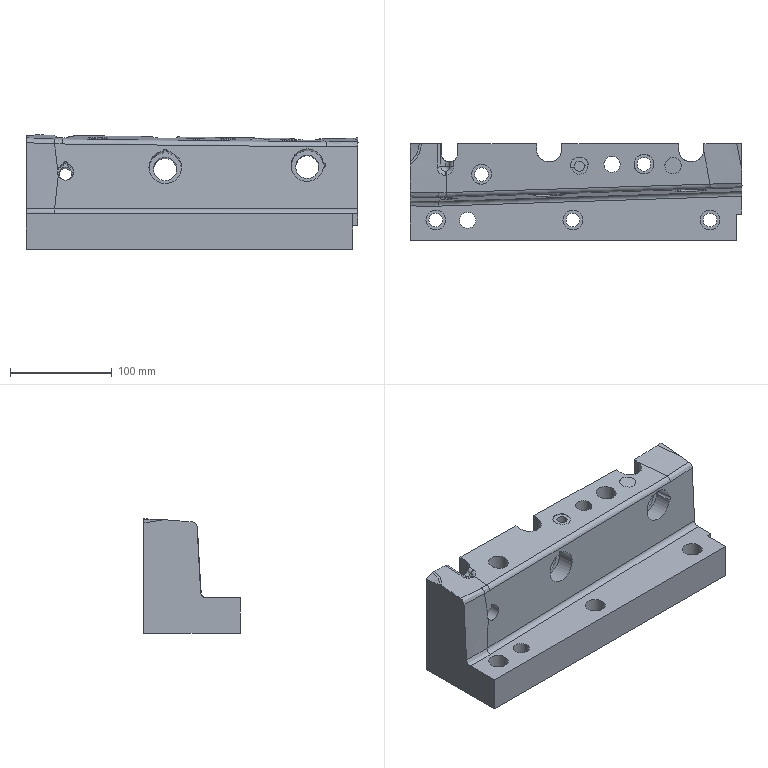Part | NX | features solid 2 | 1 solid | 79 faces | box 327 x 95 x 112.902 mm | volume 2002505 mm3 | cylinder 32 | plane 30 | spline 15 | torus 1 | sphere 1 | commonest cylinder face diameters 13.5 x5 19.5 x5 10 x4 4 x3 16 x3 23 x2